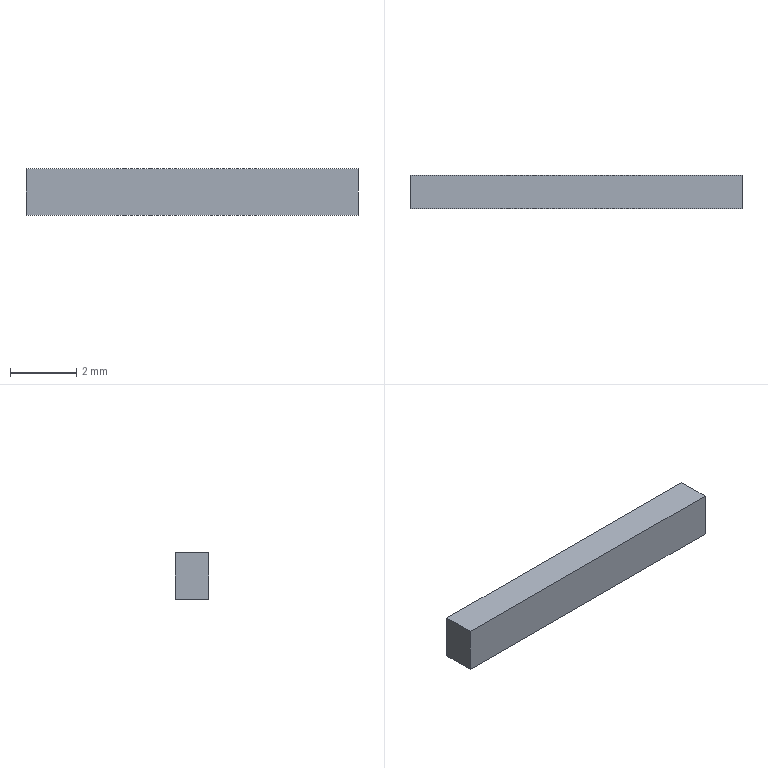Part | SolidWorks | features BaseBody 1 | 1 solid | 6 faces | box 10 x 1 x 1.4 mm | volume 14 mm3 | plane 6
STEP:
#1=CARTESIAN_POINT('',(-4.05,-20.,2.65));
#2=VERTEX_POINT('',#1);
#3=CARTESIAN_POINT('',(-4.05,-20.,1.25));
#4=VERTEX_POINT('',#3);
#5=CARTESIAN_POINT('',(-4.05,-20.,2.65));
#6=DIRECTION('',(0.,0.,-1.));
#7=VECTOR('',#6,1000.);
#8=LINE('',#5,#7);
#9=EDGE_CURVE('',#2,#4,#8,.T.);
#10=ORIENTED_EDGE('',*,*,#9,.F.);
#11=CARTESIAN_POINT('',(-4.05,-19.,2.65));
#12=VERTEX_POINT('',#11);
#13=CARTESIAN_POINT('',(-4.05,-19.,2.65));
#14=DIRECTION('',(0.,-1.,0.));
#15=VECTOR('',#14,1000.);
#16=LINE('',#13,#15);
#17=EDGE_CURVE('',#12,#2,#16,.T.);
#18=ORIENTED_EDGE('',*,*,#17,.F.);
#19=CARTESIAN_POINT('',(-4.05,-19.,1.25));
#20=VERTEX_POINT('',#19);
#21=CARTESIAN_POINT('',(-4.05,-19.,2.65));
#22=DIRECTION('',(0.,0.,-1.));
#23=VECTOR('',#22,1000.);
#24=LINE('',#21,#23);
#25=EDGE_CURVE('',#12,#20,#24,.T.);
#26=ORIENTED_EDGE('',*,*,#25,.T.);
#27=CARTESIAN_POINT('',(-4.05,-19.,1.25));
#28=DIRECTION('',(0.,-1.,0.));
#29=VECTOR('',#28,1000.);
#30=LINE('',#27,#29);
#31=EDGE_CURVE('',#20,#4,#30,.T.);
#32=ORIENTED_EDGE('',*,*,#31,.T.);
#33=EDGE_LOOP('',(#10,#18,#26,#32));
#34=FACE_OUTER_BOUND('',#33,.T.);
#35=CARTESIAN_POINT('',(-4.05,-19.,2.65));
#36=DIRECTION('',(-1.,0.,0.));
#37=DIRECTION('',(0.,0.,1.));
#38=AXIS2_PLACEMENT_3D('',#35,#36,#37);
#39=PLANE('',#38);
#40=ADVANCED_FACE('',(#34),#39,.T.);
#41=CARTESIAN_POINT('',(5.95,-20.,1.25));
#42=VERTEX_POINT('',#41);
#43=CARTESIAN_POINT('',(-4.05,-20.,1.25));
#44=DIRECTION('',(1.,0.,0.));
#45=VECTOR('',#44,1000.);
#46=LINE('',#43,#45);
#47=EDGE_CURVE('',#4,#42,#46,.T.);
#48=ORIENTED_EDGE('',*,*,#47,.F.);
#49=ORIENTED_EDGE('',*,*,#31,.F.);
#50=CARTESIAN_POINT('',(5.95,-19.,1.25));
#51=VERTEX_POINT('',#50);
#52=CARTESIAN_POINT('',(-4.05,-19.,1.25));
#53=DIRECTION('',(1.,0.,0.));
#54=VECTOR('',#53,1000.);
#55=LINE('',#52,#54);
#56=EDGE_CURVE('',#20,#51,#55,.T.);
#57=ORIENTED_EDGE('',*,*,#56,.T.);
#58=CARTESIAN_POINT('',(5.95,-19.,1.25));
#59=DIRECTION('',(0.,-1.,0.));
#60=VECTOR('',#59,1000.);
#61=LINE('',#58,#60);
#62=EDGE_CURVE('',#51,#42,#61,.T.);
#63=ORIENTED_EDGE('',*,*,#62,.T.);
#64=EDGE_LOOP('',(#48,#49,#57,#63));
#65=FACE_OUTER_BOUND('',#64,.T.);
#66=CARTESIAN_POINT('',(-4.05,-19.,1.25));
#67=DIRECTION('',(0.,0.,-1.));
#68=DIRECTION('',(-1.,0.,0.));
#69=AXIS2_PLACEMENT_3D('',#66,#67,#68);
#70=PLANE('',#69);
#71=ADVANCED_FACE('',(#65),#70,.T.);
#72=CARTESIAN_POINT('',(5.95,-20.,2.65));
#73=VERTEX_POINT('',#72);
#74=CARTESIAN_POINT('',(5.95,-20.,1.25));
#75=DIRECTION('',(0.,0.,1.));
#76=VECTOR('',#75,1000.);
#77=LINE('',#74,#76);
#78=EDGE_CURVE('',#42,#73,#77,.T.);
#79=ORIENTED_EDGE('',*,*,#78,.F.);
#80=ORIENTED_EDGE('',*,*,#62,.F.);
#81=CARTESIAN_POINT('',(5.95,-19.,2.65));
#82=VERTEX_POINT('',#81);
#83=CARTESIAN_POINT('',(5.95,-19.,1.25));
#84=DIRECTION('',(0.,0.,1.));
#85=VECTOR('',#84,1000.);
#86=LINE('',#83,#85);
#87=EDGE_CURVE('',#51,#82,#86,.T.);
#88=ORIENTED_EDGE('',*,*,#87,.T.);
#89=CARTESIAN_POINT('',(5.95,-19.,2.65));
#90=DIRECTION('',(0.,-1.,0.));
#91=VECTOR('',#90,1000.);
#92=LINE('',#89,#91);
#93=EDGE_CURVE('',#82,#73,#92,.T.);
#94=ORIENTED_EDGE('',*,*,#93,.T.);
#95=EDGE_LOOP('',(#79,#80,#88,#94));
#96=FACE_OUTER_BOUND('',#95,.T.);
#97=CARTESIAN_POINT('',(5.95,-19.,1.25));
#98=DIRECTION('',(1.,0.,0.));
#99=DIRECTION('',(0.,0.,-1.));
#100=AXIS2_PLACEMENT_3D('',#97,#98,#99);
#101=PLANE('',#100);
#102=ADVANCED_FACE('',(#96),#101,.T.);
#103=CARTESIAN_POINT('',(5.95,-20.,2.65));
#104=DIRECTION('',(-1.,0.,0.));
#105=VECTOR('',#104,1000.);
#106=LINE('',#103,#105);
#107=EDGE_CURVE('',#73,#2,#106,.T.);
#108=ORIENTED_EDGE('',*,*,#107,.F.);
#109=ORIENTED_EDGE('',*,*,#93,.F.);
#110=CARTESIAN_POINT('',(5.95,-19.,2.65));
#111=DIRECTION('',(-1.,0.,0.));
#112=VECTOR('',#111,1000.);
#113=LINE('',#110,#112);
#114=EDGE_CURVE('',#82,#12,#113,.T.);
#115=ORIENTED_EDGE('',*,*,#114,.T.);
#116=ORIENTED_EDGE('',*,*,#17,.T.);
#117=EDGE_LOOP('',(#108,#109,#115,#116));
#118=FACE_OUTER_BOUND('',#117,.T.);
#119=CARTESIAN_POINT('',(5.95,-19.,2.65));
#120=DIRECTION('',(0.,0.,1.));
#121=DIRECTION('',(1.,0.,0.));
#122=AXIS2_PLACEMENT_3D('',#119,#120,#121);
#123=PLANE('',#122);
#124=ADVANCED_FACE('',(#118),#123,.T.);
#125=ORIENTED_EDGE('',*,*,#25,.F.);
#126=ORIENTED_EDGE('',*,*,#114,.F.);
#127=ORIENTED_EDGE('',*,*,#87,.F.);
#128=ORIENTED_EDGE('',*,*,#56,.F.);
#129=EDGE_LOOP('',(#125,#126,#127,#128));
#130=FACE_OUTER_BOUND('',#129,.T.);
#131=CARTESIAN_POINT('',(0.,-19.,0.));
#132=DIRECTION('',(0.,-1.,0.));
#133=DIRECTION('',(0.,0.,-1.));
#134=AXIS2_PLACEMENT_3D('',#131,#132,#133);
#135=PLANE('',#134);
#136=ADVANCED_FACE('',(#130),#135,.F.);
#137=ORIENTED_EDGE('',*,*,#9,.T.);
#138=ORIENTED_EDGE('',*,*,#47,.T.);
#139=ORIENTED_EDGE('',*,*,#78,.T.);
#140=ORIENTED_EDGE('',*,*,#107,.T.);
#141=EDGE_LOOP('',(#137,#138,#139,#140));
#142=FACE_OUTER_BOUND('',#141,.T.);
#143=CARTESIAN_POINT('',(0.,-20.,0.));
#144=DIRECTION('',(0.,-1.,0.));
#145=DIRECTION('',(0.,0.,-1.));
#146=AXIS2_PLACEMENT_3D('',#143,#144,#145);
#147=PLANE('',#146);
#148=ADVANCED_FACE('',(#142),#147,.T.);
#149=CLOSED_SHELL('',(#40,#71,#102,#124,#136,#148));
#150=MANIFOLD_SOLID_BREP('',#149);
#151=CARTESIAN_POINT('',(0.,0.,0.));
#152=DIRECTION('',(0.,0.,1.));
#153=DIRECTION('',(1.,0.,0.));
#154=AXIS2_PLACEMENT_3D('',#151,#152,#153);
#155=(LENGTH_UNIT()NAMED_UNIT(*)SI_UNIT(.MILLI.,.METRE.));
#156=UNCERTAINTY_MEASURE_WITH_UNIT(LENGTH_MEASURE(0.00001),#155,'','');
#157=(NAMED_UNIT(*)PLANE_ANGLE_UNIT()SI_UNIT($,.RADIAN.));
#158=(NAMED_UNIT(*)SI_UNIT($,.STERADIAN.)SOLID_ANGLE_UNIT());
#159=(GEOMETRIC_REPRESENTATION_CONTEXT(3)GLOBAL_UNCERTAINTY_ASSIGNED_CONTEXT((#156))GLOBAL_UNIT_ASSIGNED_CONTEXT((#155,#157,#158))REPRESENTATION_CONTEXT('',''));
#160=ADVANCED_BREP_SHAPE_REPRESENTATION('',(#150,#154),#159);